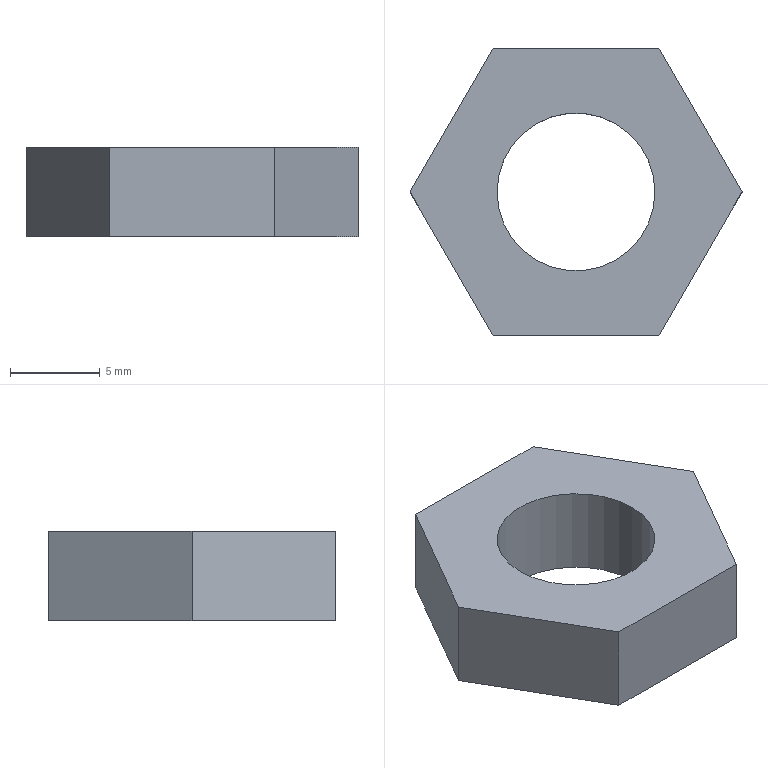Part | NX | features SKETCH 3, DATUM_CSYS 2, EXTRUDE 2, LINE 1, META 1, SYMBOLIC_THREAD 1, THREADS 1 | 1 solid | 9 faces | box 18.475 x 16 x 5 mm | volume 805.635 mm3 | plane 8 | cylinder 1 | commonest cylinder face diameters 8.782 x1
STEP:
#1=CARTESIAN_POINT('',(4.619,8.,5.));
#2=VERTEX_POINT('',#1);
#3=CARTESIAN_POINT('',(9.238,0.,5.));
#4=VERTEX_POINT('',#3);
#5=CARTESIAN_POINT('',(4.619,8.,5.));
#6=DIRECTION('',(0.5,-0.866,0.));
#7=VECTOR('',#6,1000.);
#8=LINE('',#5,#7);
#9=EDGE_CURVE('',#2,#4,#8,.T.);
#10=ORIENTED_EDGE('',*,*,#9,.F.);
#11=CARTESIAN_POINT('',(-4.619,8.,5.));
#12=VERTEX_POINT('',#11);
#13=CARTESIAN_POINT('',(-4.619,8.,5.));
#14=DIRECTION('',(1.,0.,0.));
#15=VECTOR('',#14,1000.);
#16=LINE('',#13,#15);
#17=EDGE_CURVE('',#12,#2,#16,.T.);
#18=ORIENTED_EDGE('',*,*,#17,.F.);
#19=CARTESIAN_POINT('',(-9.238,0.,5.));
#20=VERTEX_POINT('',#19);
#21=CARTESIAN_POINT('',(-9.238,0.,5.));
#22=DIRECTION('',(0.5,0.866,0.));
#23=VECTOR('',#22,1000.);
#24=LINE('',#21,#23);
#25=EDGE_CURVE('',#20,#12,#24,.T.);
#26=ORIENTED_EDGE('',*,*,#25,.F.);
#27=CARTESIAN_POINT('',(-4.619,-8.,5.));
#28=VERTEX_POINT('',#27);
#29=CARTESIAN_POINT('',(-4.619,-8.,5.));
#30=DIRECTION('',(-0.5,0.866,0.));
#31=VECTOR('',#30,1000.);
#32=LINE('',#29,#31);
#33=EDGE_CURVE('',#28,#20,#32,.T.);
#34=ORIENTED_EDGE('',*,*,#33,.F.);
#35=CARTESIAN_POINT('',(4.619,-8.,5.));
#36=VERTEX_POINT('',#35);
#37=CARTESIAN_POINT('',(4.619,-8.,5.));
#38=DIRECTION('',(-1.,0.,0.));
#39=VECTOR('',#38,1000.);
#40=LINE('',#37,#39);
#41=EDGE_CURVE('',#36,#28,#40,.T.);
#42=ORIENTED_EDGE('',*,*,#41,.F.);
#43=CARTESIAN_POINT('',(9.238,0.,5.));
#44=DIRECTION('',(-0.5,-0.866,0.));
#45=VECTOR('',#44,1000.);
#46=LINE('',#43,#45);
#47=EDGE_CURVE('',#4,#36,#46,.T.);
#48=ORIENTED_EDGE('',*,*,#47,.F.);
#49=EDGE_LOOP('',(#10,#18,#26,#34,#42,#48));
#50=FACE_BOUND('',#49,.T.);
#51=CARTESIAN_POINT('',(4.391,0.,5.));
#52=VERTEX_POINT('',#51);
#53=CARTESIAN_POINT('',(0.,0.,5.));
#54=DIRECTION('',(0.,0.,-1.));
#55=DIRECTION('',(1.,0.,0.));
#56=AXIS2_PLACEMENT_3D('',#53,#54,#55);
#57=CIRCLE('',#56,4.391);
#58=EDGE_CURVE('',#52,#52,#57,.T.);
#59=ORIENTED_EDGE('',*,*,#58,.T.);
#60=EDGE_LOOP('',(#59));
#61=FACE_BOUND('',#60,.T.);
#62=CARTESIAN_POINT('',(0.,16.,5.));
#63=DIRECTION('',(0.,0.,1.));
#64=DIRECTION('',(1.,0.,0.));
#65=AXIS2_PLACEMENT_3D('',#62,#63,#64);
#66=PLANE('',#65);
#67=ADVANCED_FACE('',(#50,#61),#66,.T.);
#68=CARTESIAN_POINT('',(4.619,8.,0.));
#69=VERTEX_POINT('',#68);
#70=CARTESIAN_POINT('',(9.238,0.,0.));
#71=VERTEX_POINT('',#70);
#72=CARTESIAN_POINT('',(4.619,8.,0.));
#73=DIRECTION('',(0.5,-0.866,0.));
#74=VECTOR('',#73,1000.);
#75=LINE('',#72,#74);
#76=EDGE_CURVE('',#69,#71,#75,.T.);
#77=ORIENTED_EDGE('',*,*,#76,.T.);
#78=CARTESIAN_POINT('',(4.619,-8.,0.));
#79=VERTEX_POINT('',#78);
#80=CARTESIAN_POINT('',(9.238,0.,0.));
#81=DIRECTION('',(-0.5,-0.866,0.));
#82=VECTOR('',#81,1000.);
#83=LINE('',#80,#82);
#84=EDGE_CURVE('',#71,#79,#83,.T.);
#85=ORIENTED_EDGE('',*,*,#84,.T.);
#86=CARTESIAN_POINT('',(-4.619,-8.,0.));
#87=VERTEX_POINT('',#86);
#88=CARTESIAN_POINT('',(4.619,-8.,0.));
#89=DIRECTION('',(-1.,0.,0.));
#90=VECTOR('',#89,1000.);
#91=LINE('',#88,#90);
#92=EDGE_CURVE('',#79,#87,#91,.T.);
#93=ORIENTED_EDGE('',*,*,#92,.T.);
#94=CARTESIAN_POINT('',(-9.238,0.,0.));
#95=VERTEX_POINT('',#94);
#96=CARTESIAN_POINT('',(-4.619,-8.,0.));
#97=DIRECTION('',(-0.5,0.866,0.));
#98=VECTOR('',#97,1000.);
#99=LINE('',#96,#98);
#100=EDGE_CURVE('',#87,#95,#99,.T.);
#101=ORIENTED_EDGE('',*,*,#100,.T.);
#102=CARTESIAN_POINT('',(-4.619,8.,0.));
#103=VERTEX_POINT('',#102);
#104=CARTESIAN_POINT('',(-9.238,0.,0.));
#105=DIRECTION('',(0.5,0.866,0.));
#106=VECTOR('',#105,1000.);
#107=LINE('',#104,#106);
#108=EDGE_CURVE('',#95,#103,#107,.T.);
#109=ORIENTED_EDGE('',*,*,#108,.T.);
#110=CARTESIAN_POINT('',(-4.619,8.,0.));
#111=DIRECTION('',(1.,0.,0.));
#112=VECTOR('',#111,1000.);
#113=LINE('',#110,#112);
#114=EDGE_CURVE('',#103,#69,#113,.T.);
#115=ORIENTED_EDGE('',*,*,#114,.T.);
#116=EDGE_LOOP('',(#77,#85,#93,#101,#109,#115));
#117=FACE_BOUND('',#116,.T.);
#118=CARTESIAN_POINT('',(4.391,0.,0.));
#119=VERTEX_POINT('',#118);
#120=CARTESIAN_POINT('',(0.,0.,0.));
#121=DIRECTION('',(0.,0.,-1.));
#122=DIRECTION('',(1.,0.,0.));
#123=AXIS2_PLACEMENT_3D('',#120,#121,#122);
#124=CIRCLE('',#123,4.391);
#125=EDGE_CURVE('',#119,#119,#124,.T.);
#126=ORIENTED_EDGE('',*,*,#125,.F.);
#127=EDGE_LOOP('',(#126));
#128=FACE_BOUND('',#127,.T.);
#129=CARTESIAN_POINT('',(0.,16.,0.));
#130=DIRECTION('',(0.,0.,1.));
#131=DIRECTION('',(1.,0.,0.));
#132=AXIS2_PLACEMENT_3D('',#129,#130,#131);
#133=PLANE('',#132);
#134=ADVANCED_FACE('',(#117,#128),#133,.F.);
#135=ORIENTED_EDGE('',*,*,#76,.F.);
#136=CARTESIAN_POINT('',(4.619,8.,5.));
#137=DIRECTION('',(0.,0.,-1.));
#138=VECTOR('',#137,1000.);
#139=LINE('',#136,#138);
#140=EDGE_CURVE('',#2,#69,#139,.T.);
#141=ORIENTED_EDGE('',*,*,#140,.F.);
#142=ORIENTED_EDGE('',*,*,#9,.T.);
#143=CARTESIAN_POINT('',(9.238,0.,5.));
#144=DIRECTION('',(0.,0.,-1.));
#145=VECTOR('',#144,1000.);
#146=LINE('',#143,#145);
#147=EDGE_CURVE('',#4,#71,#146,.T.);
#148=ORIENTED_EDGE('',*,*,#147,.T.);
#149=EDGE_LOOP('',(#135,#141,#142,#148));
#150=FACE_BOUND('',#149,.T.);
#151=CARTESIAN_POINT('',(4.619,8.,5.));
#152=DIRECTION('',(0.866,0.5,0.));
#153=DIRECTION('',(-0.5,0.866,0.));
#154=AXIS2_PLACEMENT_3D('',#151,#152,#153);
#155=PLANE('',#154);
#156=ADVANCED_FACE('',(#150),#155,.T.);
#157=ORIENTED_EDGE('',*,*,#84,.F.);
#158=ORIENTED_EDGE('',*,*,#147,.F.);
#159=ORIENTED_EDGE('',*,*,#47,.T.);
#160=CARTESIAN_POINT('',(4.619,-8.,5.));
#161=DIRECTION('',(0.,0.,-1.));
#162=VECTOR('',#161,1000.);
#163=LINE('',#160,#162);
#164=EDGE_CURVE('',#36,#79,#163,.T.);
#165=ORIENTED_EDGE('',*,*,#164,.T.);
#166=EDGE_LOOP('',(#157,#158,#159,#165));
#167=FACE_BOUND('',#166,.T.);
#168=CARTESIAN_POINT('',(9.238,0.,5.));
#169=DIRECTION('',(0.866,-0.5,0.));
#170=DIRECTION('',(0.5,0.866,0.));
#171=AXIS2_PLACEMENT_3D('',#168,#169,#170);
#172=PLANE('',#171);
#173=ADVANCED_FACE('',(#167),#172,.T.);
#174=ORIENTED_EDGE('',*,*,#92,.F.);
#175=ORIENTED_EDGE('',*,*,#164,.F.);
#176=ORIENTED_EDGE('',*,*,#41,.T.);
#177=CARTESIAN_POINT('',(-4.619,-8.,5.));
#178=DIRECTION('',(0.,0.,-1.));
#179=VECTOR('',#178,1000.);
#180=LINE('',#177,#179);
#181=EDGE_CURVE('',#28,#87,#180,.T.);
#182=ORIENTED_EDGE('',*,*,#181,.T.);
#183=EDGE_LOOP('',(#174,#175,#176,#182));
#184=FACE_BOUND('',#183,.T.);
#185=CARTESIAN_POINT('',(4.619,-8.,5.));
#186=DIRECTION('',(0.,-1.,0.));
#187=DIRECTION('',(0.,0.,-1.));
#188=AXIS2_PLACEMENT_3D('',#185,#186,#187);
#189=PLANE('',#188);
#190=ADVANCED_FACE('',(#184),#189,.T.);
#191=ORIENTED_EDGE('',*,*,#100,.F.);
#192=ORIENTED_EDGE('',*,*,#181,.F.);
#193=ORIENTED_EDGE('',*,*,#33,.T.);
#194=CARTESIAN_POINT('',(-9.238,0.,5.));
#195=DIRECTION('',(0.,0.,-1.));
#196=VECTOR('',#195,1000.);
#197=LINE('',#194,#196);
#198=EDGE_CURVE('',#20,#95,#197,.T.);
#199=ORIENTED_EDGE('',*,*,#198,.T.);
#200=EDGE_LOOP('',(#191,#192,#193,#199));
#201=FACE_BOUND('',#200,.T.);
#202=CARTESIAN_POINT('',(-4.619,-8.,5.));
#203=DIRECTION('',(-0.866,-0.5,0.));
#204=DIRECTION('',(0.5,-0.866,0.));
#205=AXIS2_PLACEMENT_3D('',#202,#203,#204);
#206=PLANE('',#205);
#207=ADVANCED_FACE('',(#201),#206,.T.);
#208=ORIENTED_EDGE('',*,*,#108,.F.);
#209=ORIENTED_EDGE('',*,*,#198,.F.);
#210=ORIENTED_EDGE('',*,*,#25,.T.);
#211=CARTESIAN_POINT('',(-4.619,8.,5.));
#212=DIRECTION('',(0.,0.,-1.));
#213=VECTOR('',#212,1000.);
#214=LINE('',#211,#213);
#215=EDGE_CURVE('',#12,#103,#214,.T.);
#216=ORIENTED_EDGE('',*,*,#215,.T.);
#217=EDGE_LOOP('',(#208,#209,#210,#216));
#218=FACE_BOUND('',#217,.T.);
#219=CARTESIAN_POINT('',(-9.238,0.,5.));
#220=DIRECTION('',(-0.866,0.5,0.));
#221=DIRECTION('',(-0.5,-0.866,0.));
#222=AXIS2_PLACEMENT_3D('',#219,#220,#221);
#223=PLANE('',#222);
#224=ADVANCED_FACE('',(#218),#223,.T.);
#225=ORIENTED_EDGE('',*,*,#114,.F.);
#226=ORIENTED_EDGE('',*,*,#215,.F.);
#227=ORIENTED_EDGE('',*,*,#17,.T.);
#228=ORIENTED_EDGE('',*,*,#140,.T.);
#229=EDGE_LOOP('',(#225,#226,#227,#228));
#230=FACE_BOUND('',#229,.T.);
#231=CARTESIAN_POINT('',(-4.619,8.,5.));
#232=DIRECTION('',(0.,1.,0.));
#233=DIRECTION('',(0.,0.,1.));
#234=AXIS2_PLACEMENT_3D('',#231,#232,#233);
#235=PLANE('',#234);
#236=ADVANCED_FACE('',(#230),#235,.T.);
#237=ORIENTED_EDGE('',*,*,#58,.F.);
#238=EDGE_LOOP('',(#237));
#239=FACE_BOUND('',#238,.T.);
#240=ORIENTED_EDGE('',*,*,#125,.T.);
#241=EDGE_LOOP('',(#240));
#242=FACE_BOUND('',#241,.T.);
#243=CARTESIAN_POINT('',(0.,0.,5.));
#244=DIRECTION('',(0.,0.,-1.));
#245=DIRECTION('',(-1.,0.,0.));
#246=AXIS2_PLACEMENT_3D('',#243,#244,#245);
#247=CYLINDRICAL_SURFACE('',#246,4.391);
#248=ADVANCED_FACE('',(#239,#242),#247,.F.);
#249=CLOSED_SHELL('',(#67,#134,#156,#173,#190,#207,#224,#236,#248));
#250=MANIFOLD_SOLID_BREP('',#249);
#251=(LENGTH_UNIT()NAMED_UNIT(*)SI_UNIT(.MILLI.,.METRE.));
#252=UNCERTAINTY_MEASURE_WITH_UNIT(LENGTH_MEASURE(0.00001),#251,'','');
#253=(NAMED_UNIT(*)PLANE_ANGLE_UNIT()SI_UNIT($,.RADIAN.));
#254=(NAMED_UNIT(*)SI_UNIT($,.STERADIAN.)SOLID_ANGLE_UNIT());
#255=(GEOMETRIC_REPRESENTATION_CONTEXT(3)GLOBAL_UNCERTAINTY_ASSIGNED_CONTEXT((#252))GLOBAL_UNIT_ASSIGNED_CONTEXT((#251,#253,#254))REPRESENTATION_CONTEXT('',''));
#256=ADVANCED_BREP_SHAPE_REPRESENTATION('',(#250),#255);